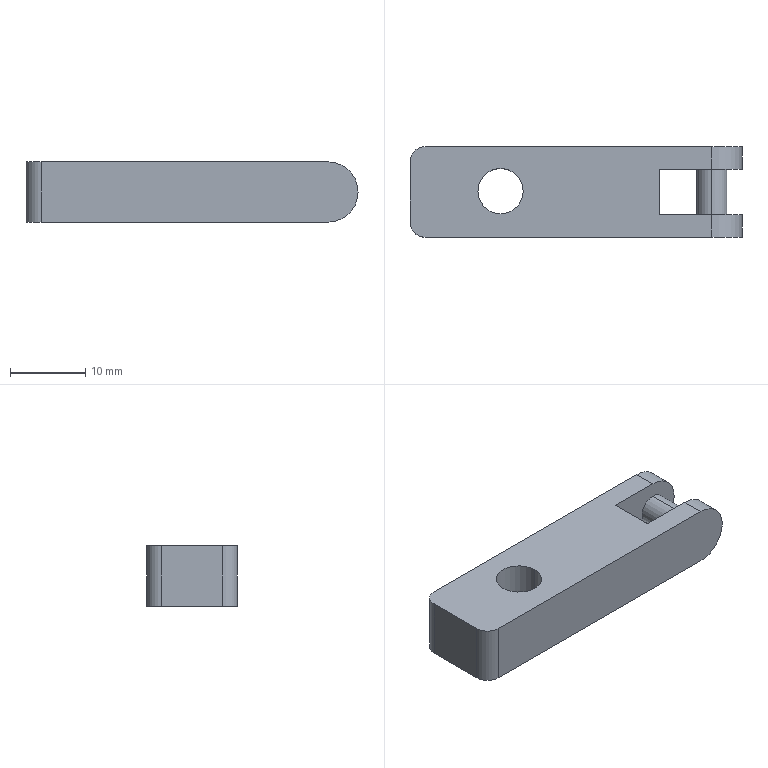Part | SolidWorks | features Extrusion 1, Fillet 1, ICE 1 | 1 solid | 18 faces | box 44 x 12 x 8 mm | volume 3492 mm3 | cylinder 10 | plane 8 | commonest cylinder face diameters 4 x4 8 x4 6 x2
STEP:
#1=CARTESIAN_POINT('',(25.743,-3.069,2.));
#2=VERTEX_POINT('',#1);
#3=CARTESIAN_POINT('',(25.743,-3.069,6.));
#4=VERTEX_POINT('',#3);
#5=CARTESIAN_POINT('',(25.743,-3.069,4.));
#6=DIRECTION('',(0.,-1.,0.));
#7=DIRECTION('',(1.,0.,0.));
#8=AXIS2_PLACEMENT_3D('',#5,#6,#7);
#9=CIRCLE('',#8,2.);
#10=EDGE_CURVE('',#2,#4,#9,.T.);
#11=ORIENTED_EDGE('',*,*,#10,.F.);
#12=CARTESIAN_POINT('',(25.743,2.931,2.));
#13=VERTEX_POINT('',#12);
#14=CARTESIAN_POINT('',(25.743,-6.069,2.));
#15=DIRECTION('',(0.,1.,0.));
#16=VECTOR('',#15,1000.);
#17=LINE('',#14,#16);
#18=EDGE_CURVE('',#2,#13,#17,.T.);
#19=ORIENTED_EDGE('',*,*,#18,.T.);
#20=CARTESIAN_POINT('',(25.743,2.931,6.));
#21=VERTEX_POINT('',#20);
#22=CARTESIAN_POINT('',(25.743,2.931,4.));
#23=DIRECTION('',(0.,1.,0.));
#24=DIRECTION('',(0.,0.,1.));
#25=AXIS2_PLACEMENT_3D('',#22,#23,#24);
#26=CIRCLE('',#25,2.);
#27=EDGE_CURVE('',#21,#13,#26,.T.);
#28=ORIENTED_EDGE('',*,*,#27,.F.);
#29=CARTESIAN_POINT('',(25.743,-6.069,6.));
#30=DIRECTION('',(0.,1.,0.));
#31=VECTOR('',#30,1000.);
#32=LINE('',#29,#31);
#33=EDGE_CURVE('',#4,#21,#32,.T.);
#34=ORIENTED_EDGE('',*,*,#33,.F.);
#35=EDGE_LOOP('',(#11,#19,#28,#34));
#36=FACE_OUTER_BOUND('',#35,.T.);
#37=CARTESIAN_POINT('',(25.743,-6.069,4.));
#38=DIRECTION('',(0.,1.,0.));
#39=DIRECTION('',(0.,0.,1.));
#40=AXIS2_PLACEMENT_3D('',#37,#38,#39);
#41=CYLINDRICAL_SURFACE('',#40,2.);
#42=ADVANCED_FACE('',(#36),#41,.T.);
#43=CARTESIAN_POINT('',(-5.257,0.03583,8.));
#44=VERTEX_POINT('',#43);
#45=CARTESIAN_POINT('',(0.743,0.03583,8.));
#46=VERTEX_POINT('',#45);
#47=CARTESIAN_POINT('',(-2.257,0.03583,8.));
#48=DIRECTION('',(0.,0.,1.));
#49=DIRECTION('',(1.,0.,0.));
#50=AXIS2_PLACEMENT_3D('',#47,#48,#49);
#51=CIRCLE('',#50,3.);
#52=EDGE_CURVE('',#44,#46,#51,.T.);
#53=ORIENTED_EDGE('',*,*,#52,.T.);
#54=CARTESIAN_POINT('',(0.743,0.03583,0.));
#55=VERTEX_POINT('',#54);
#56=CARTESIAN_POINT('',(0.743,0.03583,8.));
#57=DIRECTION('',(0.,0.,-1.));
#58=VECTOR('',#57,1000.);
#59=LINE('',#56,#58);
#60=EDGE_CURVE('',#46,#55,#59,.T.);
#61=ORIENTED_EDGE('',*,*,#60,.T.);
#62=CARTESIAN_POINT('',(-5.257,0.03583,0.));
#63=VERTEX_POINT('',#62);
#64=CARTESIAN_POINT('',(-2.257,0.03583,0.));
#65=DIRECTION('',(0.,0.,1.));
#66=DIRECTION('',(1.,0.,0.));
#67=AXIS2_PLACEMENT_3D('',#64,#65,#66);
#68=CIRCLE('',#67,3.);
#69=EDGE_CURVE('',#63,#55,#68,.T.);
#70=ORIENTED_EDGE('',*,*,#69,.F.);
#71=CARTESIAN_POINT('',(-5.257,0.03583,8.));
#72=DIRECTION('',(0.,0.,-1.));
#73=VECTOR('',#72,1000.);
#74=LINE('',#71,#73);
#75=EDGE_CURVE('',#44,#63,#74,.T.);
#76=ORIENTED_EDGE('',*,*,#75,.F.);
#77=EDGE_LOOP('',(#53,#61,#70,#76));
#78=FACE_OUTER_BOUND('',#77,.T.);
#79=CARTESIAN_POINT('',(-2.257,0.03583,8.));
#80=DIRECTION('',(0.,0.,-1.));
#81=DIRECTION('',(-1.,0.,0.));
#82=AXIS2_PLACEMENT_3D('',#79,#80,#81);
#83=CYLINDRICAL_SURFACE('',#82,3.);
#84=ADVANCED_FACE('',(#78),#83,.F.);
#85=CARTESIAN_POINT('',(-12.257,-6.069,8.));
#86=VERTEX_POINT('',#85);
#87=CARTESIAN_POINT('',(25.743,-6.069,8.));
#88=VERTEX_POINT('',#87);
#89=CARTESIAN_POINT('',(-12.257,-6.069,8.));
#90=DIRECTION('',(1.,0.,0.));
#91=VECTOR('',#90,1000.);
#92=LINE('',#89,#91);
#93=EDGE_CURVE('',#86,#88,#92,.T.);
#94=ORIENTED_EDGE('',*,*,#93,.T.);
#95=CARTESIAN_POINT('',(25.743,-3.069,8.));
#96=VERTEX_POINT('',#95);
#97=CARTESIAN_POINT('',(25.743,-3.069,8.));
#98=DIRECTION('',(0.,1.,0.));
#99=VECTOR('',#98,1000.);
#100=LINE('',#97,#99);
#101=EDGE_CURVE('',#88,#96,#100,.T.);
#102=ORIENTED_EDGE('',*,*,#101,.T.);
#103=CARTESIAN_POINT('',(18.775,-3.069,8.));
#104=VERTEX_POINT('',#103);
#105=CARTESIAN_POINT('',(18.775,-3.069,8.));
#106=DIRECTION('',(-1.,0.,0.));
#107=VECTOR('',#106,1000.);
#108=LINE('',#105,#107);
#109=EDGE_CURVE('',#96,#104,#108,.T.);
#110=ORIENTED_EDGE('',*,*,#109,.T.);
#111=CARTESIAN_POINT('',(18.775,2.931,8.));
#112=VERTEX_POINT('',#111);
#113=CARTESIAN_POINT('',(18.775,2.931,8.));
#114=DIRECTION('',(0.,1.,0.));
#115=VECTOR('',#114,1000.);
#116=LINE('',#113,#115);
#117=EDGE_CURVE('',#104,#112,#116,.T.);
#118=ORIENTED_EDGE('',*,*,#117,.T.);
#119=CARTESIAN_POINT('',(25.743,2.931,8.));
#120=VERTEX_POINT('',#119);
#121=CARTESIAN_POINT('',(18.775,2.931,8.));
#122=DIRECTION('',(1.,0.,0.));
#123=VECTOR('',#122,1000.);
#124=LINE('',#121,#123);
#125=EDGE_CURVE('',#112,#120,#124,.T.);
#126=ORIENTED_EDGE('',*,*,#125,.T.);
#127=CARTESIAN_POINT('',(25.743,5.931,8.));
#128=VERTEX_POINT('',#127);
#129=CARTESIAN_POINT('',(25.743,5.931,8.));
#130=DIRECTION('',(0.,1.,0.));
#131=VECTOR('',#130,1000.);
#132=LINE('',#129,#131);
#133=EDGE_CURVE('',#120,#128,#132,.T.);
#134=ORIENTED_EDGE('',*,*,#133,.T.);
#135=CARTESIAN_POINT('',(-12.257,5.931,8.));
#136=VERTEX_POINT('',#135);
#137=CARTESIAN_POINT('',(-12.257,5.931,8.));
#138=DIRECTION('',(-1.,0.,0.));
#139=VECTOR('',#138,1000.);
#140=LINE('',#137,#139);
#141=EDGE_CURVE('',#128,#136,#140,.T.);
#142=ORIENTED_EDGE('',*,*,#141,.T.);
#143=CARTESIAN_POINT('',(-14.257,3.931,8.));
#144=VERTEX_POINT('',#143);
#145=CARTESIAN_POINT('',(-12.257,3.931,8.));
#146=DIRECTION('',(0.,0.,1.));
#147=DIRECTION('',(1.,0.,0.));
#148=AXIS2_PLACEMENT_3D('',#145,#146,#147);
#149=CIRCLE('',#148,2.);
#150=EDGE_CURVE('',#136,#144,#149,.T.);
#151=ORIENTED_EDGE('',*,*,#150,.T.);
#152=CARTESIAN_POINT('',(-14.257,-4.069,8.));
#153=VERTEX_POINT('',#152);
#154=CARTESIAN_POINT('',(-14.257,-4.069,8.));
#155=DIRECTION('',(0.,-1.,0.));
#156=VECTOR('',#155,1000.);
#157=LINE('',#154,#156);
#158=EDGE_CURVE('',#144,#153,#157,.T.);
#159=ORIENTED_EDGE('',*,*,#158,.T.);
#160=CARTESIAN_POINT('',(-12.257,-4.069,8.));
#161=DIRECTION('',(0.,0.,1.));
#162=DIRECTION('',(1.,0.,0.));
#163=AXIS2_PLACEMENT_3D('',#160,#161,#162);
#164=CIRCLE('',#163,2.);
#165=EDGE_CURVE('',#153,#86,#164,.T.);
#166=ORIENTED_EDGE('',*,*,#165,.T.);
#167=EDGE_LOOP('',(#94,#102,#110,#118,#126,#134,#142,#151,#159,#166));
#168=FACE_OUTER_BOUND('',#167,.T.);
#169=ORIENTED_EDGE('',*,*,#52,.F.);
#170=CARTESIAN_POINT('',(-2.257,0.03583,8.));
#171=DIRECTION('',(0.,0.,1.));
#172=DIRECTION('',(1.,0.,0.));
#173=AXIS2_PLACEMENT_3D('',#170,#171,#172);
#174=CIRCLE('',#173,3.);
#175=EDGE_CURVE('',#46,#44,#174,.T.);
#176=ORIENTED_EDGE('',*,*,#175,.F.);
#177=EDGE_LOOP('',(#169,#176));
#178=FACE_BOUND('',#177,.T.);
#179=CARTESIAN_POINT('',(-12.257,3.931,8.));
#180=DIRECTION('',(0.,0.,1.));
#181=DIRECTION('',(1.,0.,0.));
#182=AXIS2_PLACEMENT_3D('',#179,#180,#181);
#183=PLANE('',#182);
#184=ADVANCED_FACE('',(#168,#178),#183,.T.);
#185=CARTESIAN_POINT('',(25.743,-3.069,0.));
#186=VERTEX_POINT('',#185);
#187=CARTESIAN_POINT('',(18.775,-3.069,0.));
#188=VERTEX_POINT('',#187);
#189=CARTESIAN_POINT('',(18.775,-3.069,0.));
#190=DIRECTION('',(-1.,0.,0.));
#191=VECTOR('',#190,1000.);
#192=LINE('',#189,#191);
#193=EDGE_CURVE('',#186,#188,#192,.T.);
#194=ORIENTED_EDGE('',*,*,#193,.F.);
#195=CARTESIAN_POINT('',(25.743,-6.069,0.));
#196=VERTEX_POINT('',#195);
#197=CARTESIAN_POINT('',(25.743,3.931,0.));
#198=DIRECTION('',(0.,-1.,0.));
#199=VECTOR('',#198,1000.);
#200=LINE('',#197,#199);
#201=EDGE_CURVE('',#186,#196,#200,.T.);
#202=ORIENTED_EDGE('',*,*,#201,.T.);
#203=CARTESIAN_POINT('',(-12.257,-6.069,0.));
#204=VERTEX_POINT('',#203);
#205=CARTESIAN_POINT('',(-12.257,-6.069,0.));
#206=DIRECTION('',(1.,0.,0.));
#207=VECTOR('',#206,1000.);
#208=LINE('',#205,#207);
#209=EDGE_CURVE('',#204,#196,#208,.T.);
#210=ORIENTED_EDGE('',*,*,#209,.F.);
#211=CARTESIAN_POINT('',(-14.257,-4.069,0.));
#212=VERTEX_POINT('',#211);
#213=CARTESIAN_POINT('',(-12.257,-4.069,0.));
#214=DIRECTION('',(0.,0.,1.));
#215=DIRECTION('',(1.,0.,0.));
#216=AXIS2_PLACEMENT_3D('',#213,#214,#215);
#217=CIRCLE('',#216,2.);
#218=EDGE_CURVE('',#212,#204,#217,.T.);
#219=ORIENTED_EDGE('',*,*,#218,.F.);
#220=CARTESIAN_POINT('',(-14.257,3.931,0.));
#221=VERTEX_POINT('',#220);
#222=CARTESIAN_POINT('',(-14.257,-4.069,0.));
#223=DIRECTION('',(0.,-1.,0.));
#224=VECTOR('',#223,1000.);
#225=LINE('',#222,#224);
#226=EDGE_CURVE('',#221,#212,#225,.T.);
#227=ORIENTED_EDGE('',*,*,#226,.F.);
#228=CARTESIAN_POINT('',(-12.257,5.931,0.));
#229=VERTEX_POINT('',#228);
#230=CARTESIAN_POINT('',(-12.257,3.931,0.));
#231=DIRECTION('',(0.,0.,1.));
#232=DIRECTION('',(1.,0.,0.));
#233=AXIS2_PLACEMENT_3D('',#230,#231,#232);
#234=CIRCLE('',#233,2.);
#235=EDGE_CURVE('',#229,#221,#234,.T.);
#236=ORIENTED_EDGE('',*,*,#235,.F.);
#237=CARTESIAN_POINT('',(25.743,5.931,0.));
#238=VERTEX_POINT('',#237);
#239=CARTESIAN_POINT('',(-12.257,5.931,0.));
#240=DIRECTION('',(-1.,0.,0.));
#241=VECTOR('',#240,1000.);
#242=LINE('',#239,#241);
#243=EDGE_CURVE('',#238,#229,#242,.T.);
#244=ORIENTED_EDGE('',*,*,#243,.F.);
#245=CARTESIAN_POINT('',(25.743,2.931,0.));
#246=VERTEX_POINT('',#245);
#247=CARTESIAN_POINT('',(25.743,3.931,0.));
#248=DIRECTION('',(0.,-1.,0.));
#249=VECTOR('',#248,1000.);
#250=LINE('',#247,#249);
#251=EDGE_CURVE('',#238,#246,#250,.T.);
#252=ORIENTED_EDGE('',*,*,#251,.T.);
#253=CARTESIAN_POINT('',(18.775,2.931,0.));
#254=VERTEX_POINT('',#253);
#255=CARTESIAN_POINT('',(18.775,2.931,0.));
#256=DIRECTION('',(1.,0.,0.));
#257=VECTOR('',#256,1000.);
#258=LINE('',#255,#257);
#259=EDGE_CURVE('',#254,#246,#258,.T.);
#260=ORIENTED_EDGE('',*,*,#259,.F.);
#261=CARTESIAN_POINT('',(18.775,2.931,0.));
#262=DIRECTION('',(0.,1.,0.));
#263=VECTOR('',#262,1000.);
#264=LINE('',#261,#263);
#265=EDGE_CURVE('',#188,#254,#264,.T.);
#266=ORIENTED_EDGE('',*,*,#265,.F.);
#267=EDGE_LOOP('',(#194,#202,#210,#219,#227,#236,#244,#252,#260,#266));
#268=FACE_OUTER_BOUND('',#267,.T.);
#269=ORIENTED_EDGE('',*,*,#69,.T.);
#270=CARTESIAN_POINT('',(-2.257,0.03583,0.));
#271=DIRECTION('',(0.,0.,1.));
#272=DIRECTION('',(1.,0.,0.));
#273=AXIS2_PLACEMENT_3D('',#270,#271,#272);
#274=CIRCLE('',#273,3.);
#275=EDGE_CURVE('',#55,#63,#274,.T.);
#276=ORIENTED_EDGE('',*,*,#275,.T.);
#277=EDGE_LOOP('',(#269,#276));
#278=FACE_BOUND('',#277,.T.);
#279=CARTESIAN_POINT('',(-12.257,3.931,0.));
#280=DIRECTION('',(0.,0.,1.));
#281=DIRECTION('',(1.,0.,0.));
#282=AXIS2_PLACEMENT_3D('',#279,#280,#281);
#283=PLANE('',#282);
#284=ADVANCED_FACE('',(#268,#278),#283,.F.);
#285=CARTESIAN_POINT('',(29.743,5.931,4.));
#286=VERTEX_POINT('',#285);
#287=CARTESIAN_POINT('',(25.743,5.931,4.));
#288=DIRECTION('',(0.,1.,0.));
#289=DIRECTION('',(0.,0.,-1.));
#290=AXIS2_PLACEMENT_3D('',#287,#288,#289);
#291=CIRCLE('',#290,4.);
#292=EDGE_CURVE('',#128,#286,#291,.T.);
#293=ORIENTED_EDGE('',*,*,#292,.T.);
#294=CARTESIAN_POINT('',(25.743,5.931,4.));
#295=DIRECTION('',(0.,1.,0.));
#296=DIRECTION('',(0.,0.,-1.));
#297=AXIS2_PLACEMENT_3D('',#294,#295,#296);
#298=CIRCLE('',#297,4.);
#299=EDGE_CURVE('',#286,#238,#298,.T.);
#300=ORIENTED_EDGE('',*,*,#299,.T.);
#301=ORIENTED_EDGE('',*,*,#243,.T.);
#302=CARTESIAN_POINT('',(-12.257,5.931,8.));
#303=DIRECTION('',(0.,0.,-1.));
#304=VECTOR('',#303,1000.);
#305=LINE('',#302,#304);
#306=EDGE_CURVE('',#136,#229,#305,.T.);
#307=ORIENTED_EDGE('',*,*,#306,.F.);
#308=ORIENTED_EDGE('',*,*,#141,.F.);
#309=EDGE_LOOP('',(#293,#300,#301,#307,#308));
#310=FACE_OUTER_BOUND('',#309,.T.);
#311=CARTESIAN_POINT('',(-12.257,5.931,8.));
#312=DIRECTION('',(0.,-1.,0.));
#313=DIRECTION('',(0.,0.,-1.));
#314=AXIS2_PLACEMENT_3D('',#311,#312,#313);
#315=PLANE('',#314);
#316=ADVANCED_FACE('',(#310),#315,.F.);
#317=ORIENTED_EDGE('',*,*,#235,.T.);
#318=CARTESIAN_POINT('',(-14.257,3.931,8.));
#319=DIRECTION('',(0.,0.,-1.));
#320=VECTOR('',#319,1000.);
#321=LINE('',#318,#320);
#322=EDGE_CURVE('',#144,#221,#321,.T.);
#323=ORIENTED_EDGE('',*,*,#322,.F.);
#324=ORIENTED_EDGE('',*,*,#150,.F.);
#325=ORIENTED_EDGE('',*,*,#306,.T.);
#326=EDGE_LOOP('',(#317,#323,#324,#325));
#327=FACE_OUTER_BOUND('',#326,.T.);
#328=CARTESIAN_POINT('',(-12.257,3.931,8.));
#329=DIRECTION('',(0.,0.,-1.));
#330=DIRECTION('',(-1.,0.,0.));
#331=AXIS2_PLACEMENT_3D('',#328,#329,#330);
#332=CYLINDRICAL_SURFACE('',#331,2.);
#333=ADVANCED_FACE('',(#327),#332,.T.);
#334=ORIENTED_EDGE('',*,*,#226,.T.);
#335=CARTESIAN_POINT('',(-14.257,-4.069,8.));
#336=DIRECTION('',(0.,0.,-1.));
#337=VECTOR('',#336,1000.);
#338=LINE('',#335,#337);
#339=EDGE_CURVE('',#153,#212,#338,.T.);
#340=ORIENTED_EDGE('',*,*,#339,.F.);
#341=ORIENTED_EDGE('',*,*,#158,.F.);
#342=ORIENTED_EDGE('',*,*,#322,.T.);
#343=EDGE_LOOP('',(#334,#340,#341,#342));
#344=FACE_OUTER_BOUND('',#343,.T.);
#345=CARTESIAN_POINT('',(-14.257,-4.069,8.));
#346=DIRECTION('',(1.,0.,0.));
#347=DIRECTION('',(0.,0.,-1.));
#348=AXIS2_PLACEMENT_3D('',#345,#346,#347);
#349=PLANE('',#348);
#350=ADVANCED_FACE('',(#344),#349,.F.);
#351=ORIENTED_EDGE('',*,*,#218,.T.);
#352=CARTESIAN_POINT('',(-12.257,-6.069,8.));
#353=DIRECTION('',(0.,0.,-1.));
#354=VECTOR('',#353,1000.);
#355=LINE('',#352,#354);
#356=EDGE_CURVE('',#86,#204,#355,.T.);
#357=ORIENTED_EDGE('',*,*,#356,.F.);
#358=ORIENTED_EDGE('',*,*,#165,.F.);
#359=ORIENTED_EDGE('',*,*,#339,.T.);
#360=EDGE_LOOP('',(#351,#357,#358,#359));
#361=FACE_OUTER_BOUND('',#360,.T.);
#362=CARTESIAN_POINT('',(-12.257,-4.069,8.));
#363=DIRECTION('',(0.,0.,-1.));
#364=DIRECTION('',(-1.,0.,0.));
#365=AXIS2_PLACEMENT_3D('',#362,#363,#364);
#366=CYLINDRICAL_SURFACE('',#365,2.);
#367=ADVANCED_FACE('',(#361),#366,.T.);
#368=ORIENTED_EDGE('',*,*,#209,.T.);
#369=CARTESIAN_POINT('',(29.743,-6.069,4.));
#370=VERTEX_POINT('',#369);
#371=CARTESIAN_POINT('',(25.743,-6.069,4.));
#372=DIRECTION('',(0.,-1.,0.));
#373=DIRECTION('',(0.,0.,1.));
#374=AXIS2_PLACEMENT_3D('',#371,#372,#373);
#375=CIRCLE('',#374,4.);
#376=EDGE_CURVE('',#196,#370,#375,.T.);
#377=ORIENTED_EDGE('',*,*,#376,.T.);
#378=CARTESIAN_POINT('',(25.743,-6.069,4.));
#379=DIRECTION('',(0.,-1.,0.));
#380=DIRECTION('',(0.,0.,1.));
#381=AXIS2_PLACEMENT_3D('',#378,#379,#380);
#382=CIRCLE('',#381,4.);
#383=EDGE_CURVE('',#370,#88,#382,.T.);
#384=ORIENTED_EDGE('',*,*,#383,.T.);
#385=ORIENTED_EDGE('',*,*,#93,.F.);
#386=ORIENTED_EDGE('',*,*,#356,.T.);
#387=EDGE_LOOP('',(#368,#377,#384,#385,#386));
#388=FACE_OUTER_BOUND('',#387,.T.);
#389=CARTESIAN_POINT('',(-12.257,-6.069,8.));
#390=DIRECTION('',(0.,1.,0.));
#391=DIRECTION('',(0.,0.,1.));
#392=AXIS2_PLACEMENT_3D('',#389,#390,#391);
#393=PLANE('',#392);
#394=ADVANCED_FACE('',(#388),#393,.F.);
#395=CARTESIAN_POINT('',(25.743,-3.069,4.));
#396=DIRECTION('',(0.,-1.,0.));
#397=DIRECTION('',(1.,0.,0.));
#398=AXIS2_PLACEMENT_3D('',#395,#396,#397);
#399=CIRCLE('',#398,2.);
#400=EDGE_CURVE('',#4,#2,#399,.T.);
#401=ORIENTED_EDGE('',*,*,#400,.T.);
#402=ORIENTED_EDGE('',*,*,#10,.T.);
#403=EDGE_LOOP('',(#401,#402));
#404=FACE_BOUND('',#403,.T.);
#405=CARTESIAN_POINT('',(29.743,-3.069,4.));
#406=VERTEX_POINT('',#405);
#407=CARTESIAN_POINT('',(25.743,-3.069,4.));
#408=DIRECTION('',(0.,1.,0.));
#409=DIRECTION('',(1.,0.,0.));
#410=AXIS2_PLACEMENT_3D('',#407,#408,#409);
#411=CIRCLE('',#410,4.);
#412=EDGE_CURVE('',#96,#406,#411,.T.);
#413=ORIENTED_EDGE('',*,*,#412,.T.);
#414=CARTESIAN_POINT('',(25.743,-3.069,4.));
#415=DIRECTION('',(0.,1.,0.));
#416=DIRECTION('',(1.,0.,0.));
#417=AXIS2_PLACEMENT_3D('',#414,#415,#416);
#418=CIRCLE('',#417,4.);
#419=EDGE_CURVE('',#406,#186,#418,.T.);
#420=ORIENTED_EDGE('',*,*,#419,.T.);
#421=ORIENTED_EDGE('',*,*,#193,.T.);
#422=CARTESIAN_POINT('',(18.775,-3.069,8.));
#423=DIRECTION('',(0.,0.,-1.));
#424=VECTOR('',#423,1000.);
#425=LINE('',#422,#424);
#426=EDGE_CURVE('',#104,#188,#425,.T.);
#427=ORIENTED_EDGE('',*,*,#426,.F.);
#428=ORIENTED_EDGE('',*,*,#109,.F.);
#429=EDGE_LOOP('',(#413,#420,#421,#427,#428));
#430=FACE_OUTER_BOUND('',#429,.T.);
#431=CARTESIAN_POINT('',(18.775,-3.069,8.));
#432=DIRECTION('',(0.,-1.,0.));
#433=DIRECTION('',(1.,0.,0.));
#434=AXIS2_PLACEMENT_3D('',#431,#432,#433);
#435=PLANE('',#434);
#436=ADVANCED_FACE('',(#404,#430),#435,.F.);
#437=ORIENTED_EDGE('',*,*,#265,.T.);
#438=CARTESIAN_POINT('',(18.775,2.931,8.));
#439=DIRECTION('',(0.,0.,-1.));
#440=VECTOR('',#439,1000.);
#441=LINE('',#438,#440);
#442=EDGE_CURVE('',#112,#254,#441,.T.);
#443=ORIENTED_EDGE('',*,*,#442,.F.);
#444=ORIENTED_EDGE('',*,*,#117,.F.);
#445=ORIENTED_EDGE('',*,*,#426,.T.);
#446=EDGE_LOOP('',(#437,#443,#444,#445));
#447=FACE_OUTER_BOUND('',#446,.T.);
#448=CARTESIAN_POINT('',(18.775,2.931,8.));
#449=DIRECTION('',(-1.,0.,0.));
#450=DIRECTION('',(0.,-1.,0.));
#451=AXIS2_PLACEMENT_3D('',#448,#449,#450);
#452=PLANE('',#451);
#453=ADVANCED_FACE('',(#447),#452,.F.);
#454=ORIENTED_EDGE('',*,*,#27,.T.);
#455=CARTESIAN_POINT('',(25.743,2.931,4.));
#456=DIRECTION('',(0.,1.,0.));
#457=DIRECTION('',(0.,0.,1.));
#458=AXIS2_PLACEMENT_3D('',#455,#456,#457);
#459=CIRCLE('',#458,2.);
#460=EDGE_CURVE('',#13,#21,#459,.T.);
#461=ORIENTED_EDGE('',*,*,#460,.T.);
#462=EDGE_LOOP('',(#454,#461));
#463=FACE_BOUND('',#462,.T.);
#464=ORIENTED_EDGE('',*,*,#259,.T.);
#465=CARTESIAN_POINT('',(29.743,2.931,4.));
#466=VERTEX_POINT('',#465);
#467=CARTESIAN_POINT('',(25.743,2.931,4.));
#468=DIRECTION('',(0.,-1.,0.));
#469=DIRECTION('',(0.,0.,1.));
#470=AXIS2_PLACEMENT_3D('',#467,#468,#469);
#471=CIRCLE('',#470,4.);
#472=EDGE_CURVE('',#246,#466,#471,.T.);
#473=ORIENTED_EDGE('',*,*,#472,.T.);
#474=CARTESIAN_POINT('',(25.743,2.931,4.));
#475=DIRECTION('',(0.,-1.,0.));
#476=DIRECTION('',(0.,0.,1.));
#477=AXIS2_PLACEMENT_3D('',#474,#475,#476);
#478=CIRCLE('',#477,4.);
#479=EDGE_CURVE('',#466,#120,#478,.T.);
#480=ORIENTED_EDGE('',*,*,#479,.T.);
#481=ORIENTED_EDGE('',*,*,#125,.F.);
#482=ORIENTED_EDGE('',*,*,#442,.T.);
#483=EDGE_LOOP('',(#464,#473,#480,#481,#482));
#484=FACE_OUTER_BOUND('',#483,.T.);
#485=CARTESIAN_POINT('',(18.775,2.931,8.));
#486=DIRECTION('',(0.,1.,0.));
#487=DIRECTION('',(0.,0.,1.));
#488=AXIS2_PLACEMENT_3D('',#485,#486,#487);
#489=PLANE('',#488);
#490=ADVANCED_FACE('',(#463,#484),#489,.F.);
#491=ORIENTED_EDGE('',*,*,#60,.F.);
#492=ORIENTED_EDGE('',*,*,#175,.T.);
#493=ORIENTED_EDGE('',*,*,#75,.T.);
#494=ORIENTED_EDGE('',*,*,#275,.F.);
#495=EDGE_LOOP('',(#491,#492,#493,#494));
#496=FACE_OUTER_BOUND('',#495,.T.);
#497=CARTESIAN_POINT('',(-2.257,0.03583,8.));
#498=DIRECTION('',(0.,0.,-1.));
#499=DIRECTION('',(-1.,0.,0.));
#500=AXIS2_PLACEMENT_3D('',#497,#498,#499);
#501=CYLINDRICAL_SURFACE('',#500,3.);
#502=ADVANCED_FACE('',(#496),#501,.F.);
#503=ORIENTED_EDGE('',*,*,#101,.F.);
#504=ORIENTED_EDGE('',*,*,#383,.F.);
#505=CARTESIAN_POINT('',(29.743,-6.069,4.));
#506=DIRECTION('',(0.,-1.,0.));
#507=VECTOR('',#506,1000.);
#508=LINE('',#505,#507);
#509=EDGE_CURVE('',#406,#370,#508,.T.);
#510=ORIENTED_EDGE('',*,*,#509,.F.);
#511=ORIENTED_EDGE('',*,*,#412,.F.);
#512=EDGE_LOOP('',(#503,#504,#510,#511));
#513=FACE_OUTER_BOUND('',#512,.T.);
#514=CARTESIAN_POINT('',(25.743,3.931,4.));
#515=DIRECTION('',(0.,-1.,0.));
#516=DIRECTION('',(0.,0.,-1.));
#517=AXIS2_PLACEMENT_3D('',#514,#515,#516);
#518=CYLINDRICAL_SURFACE('',#517,4.);
#519=ADVANCED_FACE('',(#513),#518,.T.);
#520=ORIENTED_EDGE('',*,*,#376,.F.);
#521=ORIENTED_EDGE('',*,*,#201,.F.);
#522=ORIENTED_EDGE('',*,*,#419,.F.);
#523=ORIENTED_EDGE('',*,*,#509,.T.);
#524=EDGE_LOOP('',(#520,#521,#522,#523));
#525=FACE_OUTER_BOUND('',#524,.T.);
#526=CARTESIAN_POINT('',(25.743,-6.069,4.));
#527=DIRECTION('',(0.,1.,0.));
#528=DIRECTION('',(0.,0.,1.));
#529=AXIS2_PLACEMENT_3D('',#526,#527,#528);
#530=CYLINDRICAL_SURFACE('',#529,4.);
#531=ADVANCED_FACE('',(#525),#530,.T.);
#532=ORIENTED_EDGE('',*,*,#133,.F.);
#533=ORIENTED_EDGE('',*,*,#479,.F.);
#534=CARTESIAN_POINT('',(29.743,2.931,4.));
#535=DIRECTION('',(0.,-1.,0.));
#536=VECTOR('',#535,1000.);
#537=LINE('',#534,#536);
#538=EDGE_CURVE('',#286,#466,#537,.T.);
#539=ORIENTED_EDGE('',*,*,#538,.F.);
#540=ORIENTED_EDGE('',*,*,#292,.F.);
#541=EDGE_LOOP('',(#532,#533,#539,#540));
#542=FACE_OUTER_BOUND('',#541,.T.);
#543=CARTESIAN_POINT('',(25.743,3.931,4.));
#544=DIRECTION('',(0.,-1.,0.));
#545=DIRECTION('',(0.,0.,-1.));
#546=AXIS2_PLACEMENT_3D('',#543,#544,#545);
#547=CYLINDRICAL_SURFACE('',#546,4.);
#548=ADVANCED_FACE('',(#542),#547,.T.);
#549=ORIENTED_EDGE('',*,*,#472,.F.);
#550=ORIENTED_EDGE('',*,*,#251,.F.);
#551=ORIENTED_EDGE('',*,*,#299,.F.);
#552=ORIENTED_EDGE('',*,*,#538,.T.);
#553=EDGE_LOOP('',(#549,#550,#551,#552));
#554=FACE_OUTER_BOUND('',#553,.T.);
#555=CARTESIAN_POINT('',(25.743,2.931,4.));
#556=DIRECTION('',(0.,1.,0.));
#557=DIRECTION('',(0.,0.,1.));
#558=AXIS2_PLACEMENT_3D('',#555,#556,#557);
#559=CYLINDRICAL_SURFACE('',#558,4.);
#560=ADVANCED_FACE('',(#554),#559,.T.);
#561=ORIENTED_EDGE('',*,*,#18,.F.);
#562=ORIENTED_EDGE('',*,*,#400,.F.);
#563=ORIENTED_EDGE('',*,*,#33,.T.);
#564=ORIENTED_EDGE('',*,*,#460,.F.);
#565=EDGE_LOOP('',(#561,#562,#563,#564));
#566=FACE_OUTER_BOUND('',#565,.T.);
#567=CARTESIAN_POINT('',(25.743,-6.069,4.));
#568=DIRECTION('',(0.,1.,0.));
#569=DIRECTION('',(0.,0.,1.));
#570=AXIS2_PLACEMENT_3D('',#567,#568,#569);
#571=CYLINDRICAL_SURFACE('',#570,2.);
#572=ADVANCED_FACE('',(#566),#571,.T.);
#573=CLOSED_SHELL('',(#42,#84,#184,#284,#316,#333,#350,#367,#394,#436,#453,#490,#502,#519,#531,#548,#560,#572));
#574=MANIFOLD_SOLID_BREP('',#573);
#575=CARTESIAN_POINT('',(0.,0.,0.));
#576=DIRECTION('',(0.,0.,1.));
#577=DIRECTION('',(1.,0.,0.));
#578=AXIS2_PLACEMENT_3D('',#575,#576,#577);
#579=(LENGTH_UNIT()NAMED_UNIT(*)SI_UNIT(.MILLI.,.METRE.));
#580=UNCERTAINTY_MEASURE_WITH_UNIT(LENGTH_MEASURE(0.00001),#579,'','');
#581=(NAMED_UNIT(*)PLANE_ANGLE_UNIT()SI_UNIT($,.RADIAN.));
#582=(NAMED_UNIT(*)SI_UNIT($,.STERADIAN.)SOLID_ANGLE_UNIT());
#583=(GEOMETRIC_REPRESENTATION_CONTEXT(3)GLOBAL_UNCERTAINTY_ASSIGNED_CONTEXT((#580))GLOBAL_UNIT_ASSIGNED_CONTEXT((#579,#581,#582))REPRESENTATION_CONTEXT('',''));
#584=ADVANCED_BREP_SHAPE_REPRESENTATION('',(#574,#578),#583);